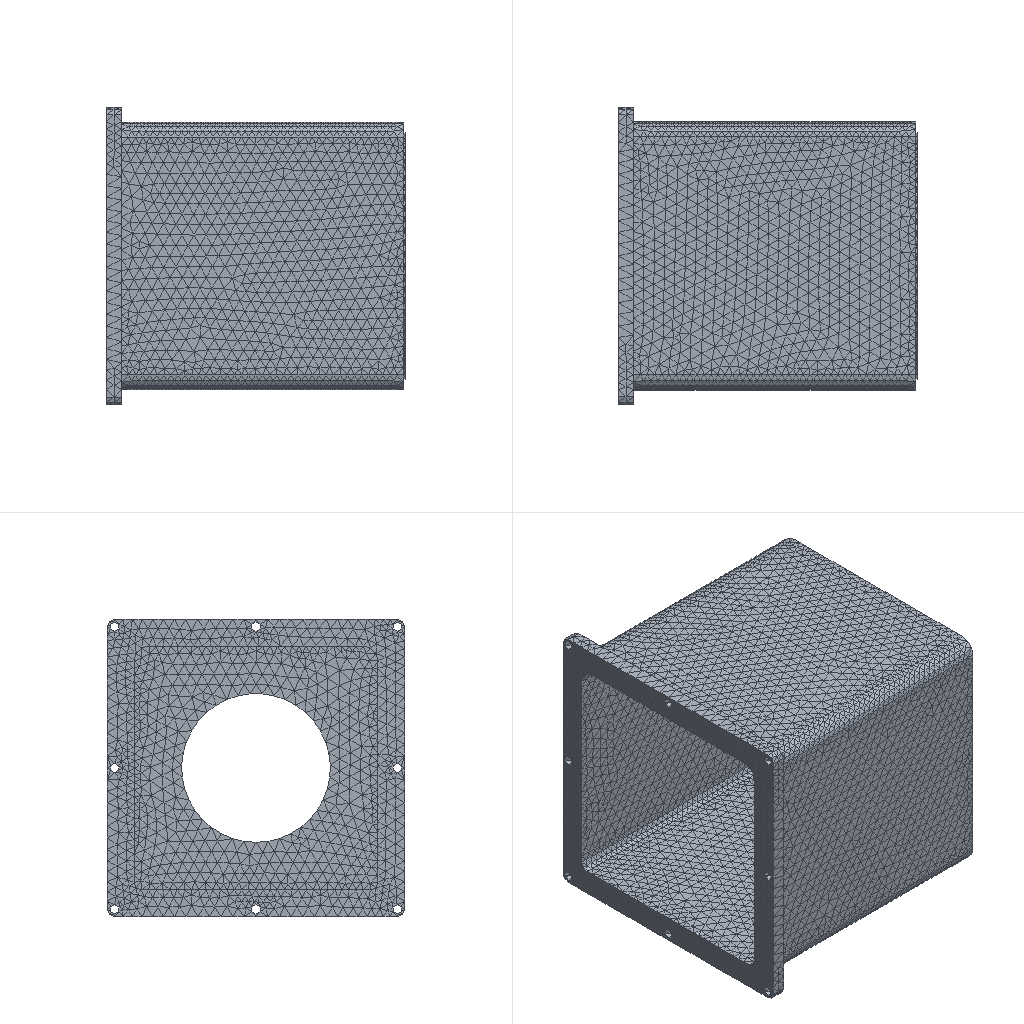Simulation study | nx simcenter
Set-up summary:
category,name,step,type,value,unit,region
solver,nx_nastran (Simcenter)
units,not stated in the deck,,not stated
analysis,deck,,static,static
analysis,solution,,SOL,101
load_step,SUBCASE 1,1,SUBCASE,SPC=1 LOAD=2
load_step,requested,,,1
mesh,nodes,,,53639
mesh,elements,,,27676
element_type,CTETRA,,solid,27676
load,nodal force total,,FX,-1500000.019,model units
load,nodal force total,,FY,0.0,model units
load,nodal force total,,FZ,0.0,model units
load,load commands in deck,,count,868
bc,support commands in deck,,count,1900
analysis,NX solution 0,,Structural,Linear Statics - Single Constraint
check,setup vs results,,match,every grid point's frame and coordinates and every element id; grid points of CTETRA elements
Nastran input file, long lists of numbers shortened:
$*$$$$$$$$$$$$$$$$$$$$$$$$$$$$$$$$$$$$$$$$$$$$$$$$$$$$$$$$$$$$$$$$$
$*
$*                    NX v10.0.0.24 TRANSLATOR
$*                    FOR NX NASTRAN VERSION 10.0
$ (33 more lines like these left out)
ASSIGN OUTPUT2='134_sim1-solution_1.op2' UNIT=12
$*
$*$$$$$$$$$$$$$$$$$$$$$$$$$$$$$$$$$$$
$*
$* EXECUTIVE CONTROL
$*
$*$$$$$$$$$$$$$$$$$$$$$$$$$$$$$$$$$$$
$*
ID,NASTRAN,134_sim1-solution_1
SOL 101
CEND
$*
$*$$$$$$$$$$$$$$$$$$$$$$$$$$$$$$$$$$$
$*
$* CASE CONTROL
$*
$*$$$$$$$$$$$$$$$$$$$$$$$$$$$$$$$$$$$
$*
TITLE = Solution 1
ECHO = NONE
SPC = 1
OUTPUT
BCRESULTS(TRACTION,FORCE,PLOT) = ALL
DISPLACEMENT(PLOT) = ALL
ESE(PLOT) = ALL
FORCE(PLOT,CORNER) = ALL
OLOAD(PLOT) = ALL
SPCFORCES(PLOT) = ALL
STRAIN(PLOT,FIBER,CORNER) = ALL
STRESS(PLOT,CORNER) = ALL
$*  NX Step: Subcase - Static Loads 1
SUBCASE 1
LABEL = Subcase - Static Loads 1
LOAD = 2
$*
$*$$$$$$$$$$$$$$$$$$$$$$$$$$$$$$$$$$$
$*
$* BULK DATA
$*
$*$$$$$$$$$$$$$$$$$$$$$$$$$$$$$$$$$$$
$*
BEGIN BULK
$*
$* PARAM CARDS
$*
PARAM      K6ROT100.0000
PARAM     OIBULK     YES
PARAM    OMACHPR     YES
PARAM       POST      -2
PARAM    POSTEXT     YES
PARAM    UNITSYS   MN-MM
$*
$* GRID CARDS
$*
GRID*              53572               00.0000000000E+00-1.000000000E+02+
*       9.5000000000E+01               0
GRID*              53573               00.0000000000E+00-1.000000000E+02+
*       -9.500000000E+01               0
$ (107274 more lines like these left out)
$*
$* ELEMENT CARDS
$*
$*  NX Mesh Collector: Solid(1)
$*  NX Mesh: 3d_mesh(1)
CTETRA         1       1       1       2   20780   20781     600     601+
+            602     603     604   21581
CTETRA         2       1       1   20782   20780   50488     605   21584+
+            602     606   21590   21591
$ (55348 more lines like these left out)
$*
$* PROPERTY CARDS
$*
$*  NX Property: PSOLID1
PSOLID         1       1       0                           SMECH
$*
$* MATERIAL CARDS
$*
$*  NX Material: Aluminum_5086
MAT1           17.2000+7        0.3300002.6600-62.5000-5
$*
$* LOAD AND CONSTRAINT CARDS
$*
$*  NX Load and Constraint: Fixed(1)
SPC            1   20604  123456  0.0000
SPC            1   20605  123456  0.0000
SPC            1   20606  123456  0.0000
SPC            1   20607  123456  0.0000
$ (1896 more lines like these left out)
$*  NX Load and Constraint: Force(1)
FORCE          2   49362       0 1631.19-1.00000  0.0000  0.0000
FORCE          2   49363       0 1703.46-1.00000  0.0000  0.0000
FORCE          2   49364       0 1684.22-1.00000  0.0000  0.0000
FORCE          2   49365       0 1670.58-1.00000  0.0000  0.0000
$ (864 more lines like these left out)
ENDDATA 0a5fb9a2
Results summary:
result,analysis,,,static
result,last_loadstep,,,1
result,primary field,,,displacements
result,reaction total,,FX,1499998.75,model units
result,reaction total,,FY,-0.01811,model units
result,reaction total,,FZ,-0.004223,model units
result,NX solution 0,,loadcases,1,mm